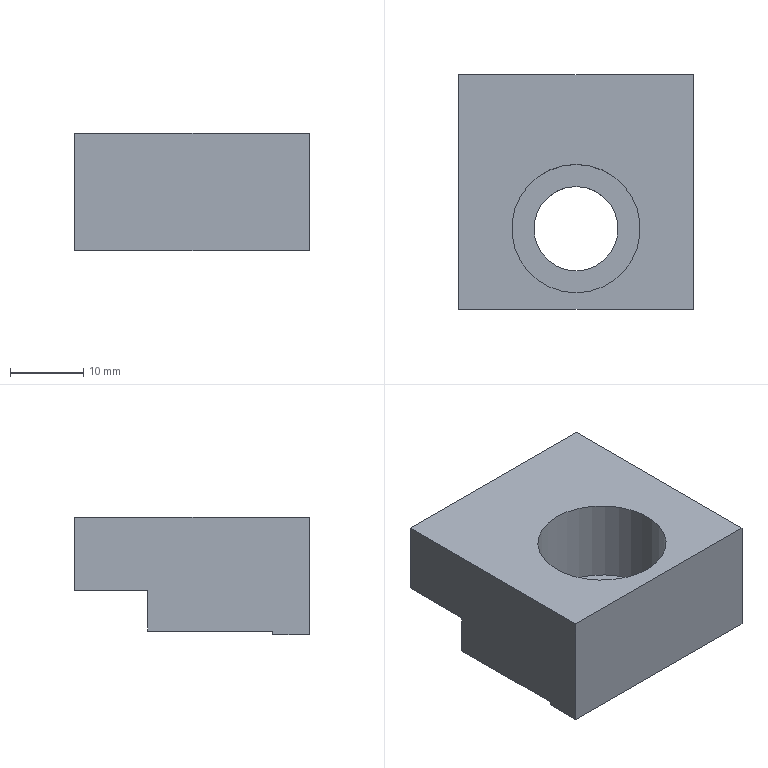Part | NX | features MAIN_BODY 2 | 1 solid | 13 faces | box 32 x 32 x 16 mm | volume 11010 mm3 | plane 11 | cylinder 2 | commonest cylinder face diameters 11.5 x1 17.5 x1
STEP:
#1=CARTESIAN_POINT('',(-279.,-369.5,260.));
#2=VERTEX_POINT('',#1);
#3=CARTESIAN_POINT('',(-279.,-369.5,276.));
#4=VERTEX_POINT('',#3);
#5=CARTESIAN_POINT('',(-279.,-369.5,260.));
#6=DIRECTION('',(0.,0.,-1.));
#7=VECTOR('',#6,1000.);
#8=LINE('',#5,#7);
#9=EDGE_CURVE('',#2,#4,#8,.F.);
#10=ORIENTED_EDGE('',*,*,#9,.F.);
#11=CARTESIAN_POINT('',(-279.,-364.5,260.));
#12=VERTEX_POINT('',#11);
#13=CARTESIAN_POINT('',(-279.,-357.5,260.));
#14=DIRECTION('',(0.,1.,0.));
#15=VECTOR('',#14,1000.);
#16=LINE('',#13,#15);
#17=EDGE_CURVE('',#2,#12,#16,.T.);
#18=ORIENTED_EDGE('',*,*,#17,.T.);
#19=CARTESIAN_POINT('',(-279.,-364.5,260.5));
#20=VERTEX_POINT('',#19);
#21=CARTESIAN_POINT('',(-279.,-364.5,260.));
#22=DIRECTION('',(0.,0.,-1.));
#23=VECTOR('',#22,1000.);
#24=LINE('',#21,#23);
#25=EDGE_CURVE('',#12,#20,#24,.F.);
#26=ORIENTED_EDGE('',*,*,#25,.T.);
#27=CARTESIAN_POINT('',(-279.,-347.5,260.5));
#28=VERTEX_POINT('',#27);
#29=CARTESIAN_POINT('',(-279.,-347.5,260.5));
#30=DIRECTION('',(0.,1.,0.));
#31=VECTOR('',#30,1000.);
#32=LINE('',#29,#31);
#33=EDGE_CURVE('',#28,#20,#32,.F.);
#34=ORIENTED_EDGE('',*,*,#33,.F.);
#35=CARTESIAN_POINT('',(-279.,-347.5,266.));
#36=VERTEX_POINT('',#35);
#37=CARTESIAN_POINT('',(-279.,-347.5,260.));
#38=DIRECTION('',(0.,0.,-1.));
#39=VECTOR('',#38,1000.);
#40=LINE('',#37,#39);
#41=EDGE_CURVE('',#28,#36,#40,.F.);
#42=ORIENTED_EDGE('',*,*,#41,.T.);
#43=CARTESIAN_POINT('',(-279.,-337.5,266.));
#44=VERTEX_POINT('',#43);
#45=CARTESIAN_POINT('',(-279.,-357.5,266.));
#46=DIRECTION('',(0.,-1.,0.));
#47=VECTOR('',#46,1000.);
#48=LINE('',#45,#47);
#49=EDGE_CURVE('',#44,#36,#48,.T.);
#50=ORIENTED_EDGE('',*,*,#49,.F.);
#51=CARTESIAN_POINT('',(-279.,-337.5,276.));
#52=VERTEX_POINT('',#51);
#53=CARTESIAN_POINT('',(-279.,-337.5,260.));
#54=DIRECTION('',(0.,0.,-1.));
#55=VECTOR('',#54,1000.);
#56=LINE('',#53,#55);
#57=EDGE_CURVE('',#44,#52,#56,.F.);
#58=ORIENTED_EDGE('',*,*,#57,.T.);
#59=CARTESIAN_POINT('',(-279.,-357.5,276.));
#60=DIRECTION('',(0.,-1.,0.));
#61=VECTOR('',#60,1000.);
#62=LINE('',#59,#61);
#63=EDGE_CURVE('',#4,#52,#62,.F.);
#64=ORIENTED_EDGE('',*,*,#63,.F.);
#65=EDGE_LOOP('',(#10,#18,#26,#34,#42,#50,#58,#64));
#66=FACE_BOUND('',#65,.T.);
#67=CARTESIAN_POINT('',(-279.,-357.5,260.));
#68=DIRECTION('',(1.,0.,0.));
#69=DIRECTION('',(0.,0.,1.));
#70=AXIS2_PLACEMENT_3D('',#67,#68,#69);
#71=PLANE('',#70);
#72=ADVANCED_FACE('',(#66),#71,.T.);
#73=CARTESIAN_POINT('',(-311.,-369.5,276.));
#74=VERTEX_POINT('',#73);
#75=CARTESIAN_POINT('',(-311.,-337.5,276.));
#76=VERTEX_POINT('',#75);
#77=CARTESIAN_POINT('',(-311.,-357.5,276.));
#78=DIRECTION('',(0.,1.,0.));
#79=VECTOR('',#78,1000.);
#80=LINE('',#77,#79);
#81=EDGE_CURVE('',#74,#76,#80,.T.);
#82=ORIENTED_EDGE('',*,*,#81,.T.);
#83=CARTESIAN_POINT('',(-311.,-337.5,266.));
#84=VERTEX_POINT('',#83);
#85=CARTESIAN_POINT('',(-311.,-337.5,260.));
#86=DIRECTION('',(0.,0.,1.));
#87=VECTOR('',#86,1000.);
#88=LINE('',#85,#87);
#89=EDGE_CURVE('',#84,#76,#88,.T.);
#90=ORIENTED_EDGE('',*,*,#89,.F.);
#91=CARTESIAN_POINT('',(-311.,-347.5,266.));
#92=VERTEX_POINT('',#91);
#93=CARTESIAN_POINT('',(-311.,-337.5,266.));
#94=DIRECTION('',(0.,1.,0.));
#95=VECTOR('',#94,1000.);
#96=LINE('',#93,#95);
#97=EDGE_CURVE('',#84,#92,#96,.F.);
#98=ORIENTED_EDGE('',*,*,#97,.T.);
#99=CARTESIAN_POINT('',(-311.,-347.5,260.5));
#100=VERTEX_POINT('',#99);
#101=CARTESIAN_POINT('',(-311.,-347.5,260.));
#102=DIRECTION('',(0.,0.,1.));
#103=VECTOR('',#102,1000.);
#104=LINE('',#101,#103);
#105=EDGE_CURVE('',#100,#92,#104,.T.);
#106=ORIENTED_EDGE('',*,*,#105,.F.);
#107=CARTESIAN_POINT('',(-311.,-364.5,260.5));
#108=VERTEX_POINT('',#107);
#109=CARTESIAN_POINT('',(-311.,-357.5,260.5));
#110=DIRECTION('',(0.,-1.,0.));
#111=VECTOR('',#110,1000.);
#112=LINE('',#109,#111);
#113=EDGE_CURVE('',#100,#108,#112,.T.);
#114=ORIENTED_EDGE('',*,*,#113,.T.);
#115=CARTESIAN_POINT('',(-311.,-364.5,260.));
#116=VERTEX_POINT('',#115);
#117=CARTESIAN_POINT('',(-311.,-364.5,260.));
#118=DIRECTION('',(0.,0.,1.));
#119=VECTOR('',#118,1000.);
#120=LINE('',#117,#119);
#121=EDGE_CURVE('',#116,#108,#120,.T.);
#122=ORIENTED_EDGE('',*,*,#121,.F.);
#123=CARTESIAN_POINT('',(-311.,-369.5,260.));
#124=VERTEX_POINT('',#123);
#125=CARTESIAN_POINT('',(-311.,-357.5,260.));
#126=DIRECTION('',(0.,-1.,0.));
#127=VECTOR('',#126,1000.);
#128=LINE('',#125,#127);
#129=EDGE_CURVE('',#124,#116,#128,.F.);
#130=ORIENTED_EDGE('',*,*,#129,.F.);
#131=CARTESIAN_POINT('',(-311.,-369.5,260.));
#132=DIRECTION('',(0.,0.,1.));
#133=VECTOR('',#132,1000.);
#134=LINE('',#131,#133);
#135=EDGE_CURVE('',#124,#74,#134,.T.);
#136=ORIENTED_EDGE('',*,*,#135,.T.);
#137=EDGE_LOOP('',(#82,#90,#98,#106,#114,#122,#130,#136));
#138=FACE_BOUND('',#137,.T.);
#139=CARTESIAN_POINT('',(-311.,-357.5,260.));
#140=DIRECTION('',(1.,0.,0.));
#141=DIRECTION('',(0.,0.,1.));
#142=AXIS2_PLACEMENT_3D('',#139,#140,#141);
#143=PLANE('',#142);
#144=ADVANCED_FACE('',(#138),#143,.F.);
#145=ORIENTED_EDGE('',*,*,#41,.F.);
#146=CARTESIAN_POINT('',(-305.,-347.5,260.5));
#147=DIRECTION('',(1.,0.,0.));
#148=VECTOR('',#147,1000.);
#149=LINE('',#146,#148);
#150=EDGE_CURVE('',#100,#28,#149,.T.);
#151=ORIENTED_EDGE('',*,*,#150,.F.);
#152=ORIENTED_EDGE('',*,*,#105,.T.);
#153=CARTESIAN_POINT('',(-305.,-347.5,266.));
#154=DIRECTION('',(-1.,0.,0.));
#155=VECTOR('',#154,1000.);
#156=LINE('',#153,#155);
#157=EDGE_CURVE('',#92,#36,#156,.F.);
#158=ORIENTED_EDGE('',*,*,#157,.T.);
#159=EDGE_LOOP('',(#145,#151,#152,#158));
#160=FACE_BOUND('',#159,.T.);
#161=CARTESIAN_POINT('',(-305.,-347.5,260.));
#162=DIRECTION('',(0.,-1.,0.));
#163=DIRECTION('',(0.,0.,-1.));
#164=AXIS2_PLACEMENT_3D('',#161,#162,#163);
#165=PLANE('',#164);
#166=ADVANCED_FACE('',(#160),#165,.F.);
#167=ORIENTED_EDGE('',*,*,#129,.T.);
#168=CARTESIAN_POINT('',(-305.,-364.5,260.));
#169=DIRECTION('',(-1.,0.,0.));
#170=VECTOR('',#169,1000.);
#171=LINE('',#168,#170);
#172=EDGE_CURVE('',#116,#12,#171,.F.);
#173=ORIENTED_EDGE('',*,*,#172,.T.);
#174=ORIENTED_EDGE('',*,*,#17,.F.);
#175=CARTESIAN_POINT('',(-305.,-369.5,260.));
#176=DIRECTION('',(-1.,0.,0.));
#177=VECTOR('',#176,1000.);
#178=LINE('',#175,#177);
#179=EDGE_CURVE('',#124,#2,#178,.F.);
#180=ORIENTED_EDGE('',*,*,#179,.F.);
#181=EDGE_LOOP('',(#167,#173,#174,#180));
#182=FACE_BOUND('',#181,.T.);
#183=CARTESIAN_POINT('',(-305.,-357.5,260.));
#184=DIRECTION('',(0.,0.,-1.));
#185=DIRECTION('',(1.,0.,0.));
#186=AXIS2_PLACEMENT_3D('',#183,#184,#185);
#187=PLANE('',#186);
#188=ADVANCED_FACE('',(#182),#187,.T.);
#189=CARTESIAN_POINT('',(-295.,-367.25,276.));
#190=VERTEX_POINT('',#189);
#191=CARTESIAN_POINT('',(-295.,-358.5,276.));
#192=DIRECTION('',(0.,0.,1.));
#193=DIRECTION('',(0.,-1.,0.));
#194=AXIS2_PLACEMENT_3D('',#191,#192,#193);
#195=CIRCLE('',#194,8.75);
#196=EDGE_CURVE('',#190,#190,#195,.T.);
#197=ORIENTED_EDGE('',*,*,#196,.F.);
#198=EDGE_LOOP('',(#197));
#199=FACE_BOUND('',#198,.T.);
#200=CARTESIAN_POINT('',(-305.,-337.5,276.));
#201=DIRECTION('',(1.,0.,0.));
#202=VECTOR('',#201,1000.);
#203=LINE('',#200,#202);
#204=EDGE_CURVE('',#76,#52,#203,.T.);
#205=ORIENTED_EDGE('',*,*,#204,.F.);
#206=ORIENTED_EDGE('',*,*,#81,.F.);
#207=CARTESIAN_POINT('',(-305.,-369.5,276.));
#208=DIRECTION('',(1.,0.,0.));
#209=VECTOR('',#208,1000.);
#210=LINE('',#207,#209);
#211=EDGE_CURVE('',#74,#4,#210,.T.);
#212=ORIENTED_EDGE('',*,*,#211,.T.);
#213=ORIENTED_EDGE('',*,*,#63,.T.);
#214=EDGE_LOOP('',(#205,#206,#212,#213));
#215=FACE_BOUND('',#214,.T.);
#216=CARTESIAN_POINT('',(-305.,-357.5,276.));
#217=DIRECTION('',(0.,0.,-1.));
#218=DIRECTION('',(1.,0.,0.));
#219=AXIS2_PLACEMENT_3D('',#216,#217,#218);
#220=PLANE('',#219);
#221=ADVANCED_FACE('',(#199,#215),#220,.F.);
#222=CARTESIAN_POINT('',(-305.,-337.5,266.));
#223=DIRECTION('',(-1.,0.,0.));
#224=VECTOR('',#223,1000.);
#225=LINE('',#222,#224);
#226=EDGE_CURVE('',#84,#44,#225,.F.);
#227=ORIENTED_EDGE('',*,*,#226,.F.);
#228=ORIENTED_EDGE('',*,*,#89,.T.);
#229=ORIENTED_EDGE('',*,*,#204,.T.);
#230=ORIENTED_EDGE('',*,*,#57,.F.);
#231=EDGE_LOOP('',(#227,#228,#229,#230));
#232=FACE_BOUND('',#231,.T.);
#233=CARTESIAN_POINT('',(-305.,-337.5,260.));
#234=DIRECTION('',(0.,-1.,0.));
#235=DIRECTION('',(0.,0.,-1.));
#236=AXIS2_PLACEMENT_3D('',#233,#234,#235);
#237=PLANE('',#236);
#238=ADVANCED_FACE('',(#232),#237,.F.);
#239=ORIENTED_EDGE('',*,*,#211,.F.);
#240=ORIENTED_EDGE('',*,*,#135,.F.);
#241=ORIENTED_EDGE('',*,*,#179,.T.);
#242=ORIENTED_EDGE('',*,*,#9,.T.);
#243=EDGE_LOOP('',(#239,#240,#241,#242));
#244=FACE_BOUND('',#243,.T.);
#245=CARTESIAN_POINT('',(-305.,-369.5,260.));
#246=DIRECTION('',(0.,-1.,0.));
#247=DIRECTION('',(0.,0.,-1.));
#248=AXIS2_PLACEMENT_3D('',#245,#246,#247);
#249=PLANE('',#248);
#250=ADVANCED_FACE('',(#244),#249,.T.);
#251=ORIENTED_EDGE('',*,*,#157,.F.);
#252=ORIENTED_EDGE('',*,*,#97,.F.);
#253=ORIENTED_EDGE('',*,*,#226,.T.);
#254=ORIENTED_EDGE('',*,*,#49,.T.);
#255=EDGE_LOOP('',(#251,#252,#253,#254));
#256=FACE_BOUND('',#255,.T.);
#257=CARTESIAN_POINT('',(-305.,-337.5,266.));
#258=DIRECTION('',(0.,0.,-1.));
#259=DIRECTION('',(1.,0.,0.));
#260=AXIS2_PLACEMENT_3D('',#257,#258,#259);
#261=PLANE('',#260);
#262=ADVANCED_FACE('',(#256),#261,.T.);
#263=CARTESIAN_POINT('',(-295.,-364.25,260.5));
#264=VERTEX_POINT('',#263);
#265=CARTESIAN_POINT('',(-295.,-358.5,260.5));
#266=DIRECTION('',(0.,0.,1.));
#267=DIRECTION('',(0.,-1.,0.));
#268=AXIS2_PLACEMENT_3D('',#265,#266,#267);
#269=CIRCLE('',#268,5.75);
#270=EDGE_CURVE('',#264,#264,#269,.T.);
#271=ORIENTED_EDGE('',*,*,#270,.T.);
#272=EDGE_LOOP('',(#271));
#273=FACE_BOUND('',#272,.T.);
#274=ORIENTED_EDGE('',*,*,#33,.T.);
#275=CARTESIAN_POINT('',(-305.,-364.5,260.5));
#276=DIRECTION('',(1.,0.,0.));
#277=VECTOR('',#276,1000.);
#278=LINE('',#275,#277);
#279=EDGE_CURVE('',#108,#20,#278,.T.);
#280=ORIENTED_EDGE('',*,*,#279,.F.);
#281=ORIENTED_EDGE('',*,*,#113,.F.);
#282=ORIENTED_EDGE('',*,*,#150,.T.);
#283=EDGE_LOOP('',(#274,#280,#281,#282));
#284=FACE_BOUND('',#283,.T.);
#285=CARTESIAN_POINT('',(-305.,-347.5,260.5));
#286=DIRECTION('',(0.,0.,-1.));
#287=DIRECTION('',(1.,0.,0.));
#288=AXIS2_PLACEMENT_3D('',#285,#286,#287);
#289=PLANE('',#288);
#290=ADVANCED_FACE('',(#273,#284),#289,.T.);
#291=ORIENTED_EDGE('',*,*,#172,.F.);
#292=ORIENTED_EDGE('',*,*,#121,.T.);
#293=ORIENTED_EDGE('',*,*,#279,.T.);
#294=ORIENTED_EDGE('',*,*,#25,.F.);
#295=EDGE_LOOP('',(#291,#292,#293,#294));
#296=FACE_BOUND('',#295,.T.);
#297=CARTESIAN_POINT('',(-305.,-364.5,260.));
#298=DIRECTION('',(0.,-1.,0.));
#299=DIRECTION('',(0.,0.,-1.));
#300=AXIS2_PLACEMENT_3D('',#297,#298,#299);
#301=PLANE('',#300);
#302=ADVANCED_FACE('',(#296),#301,.F.);
#303=ORIENTED_EDGE('',*,*,#270,.F.);
#304=EDGE_LOOP('',(#303));
#305=FACE_BOUND('',#304,.T.);
#306=CARTESIAN_POINT('',(-295.,-364.25,264.5));
#307=VERTEX_POINT('',#306);
#308=CARTESIAN_POINT('',(-295.,-358.5,264.5));
#309=DIRECTION('',(0.,0.,1.));
#310=DIRECTION('',(0.,-1.,0.));
#311=AXIS2_PLACEMENT_3D('',#308,#309,#310);
#312=CIRCLE('',#311,5.75);
#313=EDGE_CURVE('',#307,#307,#312,.T.);
#314=ORIENTED_EDGE('',*,*,#313,.T.);
#315=EDGE_LOOP('',(#314));
#316=FACE_BOUND('',#315,.T.);
#317=CARTESIAN_POINT('',(-295.,-358.5,226.));
#318=DIRECTION('',(0.,0.,-1.));
#319=DIRECTION('',(0.,-1.,0.));
#320=AXIS2_PLACEMENT_3D('',#317,#318,#319);
#321=CYLINDRICAL_SURFACE('',#320,5.75);
#322=ADVANCED_FACE('',(#305,#316),#321,.F.);
#323=ORIENTED_EDGE('',*,*,#313,.F.);
#324=EDGE_LOOP('',(#323));
#325=FACE_BOUND('',#324,.T.);
#326=CARTESIAN_POINT('',(-295.,-367.25,264.5));
#327=VERTEX_POINT('',#326);
#328=CARTESIAN_POINT('',(-295.,-358.5,264.5));
#329=DIRECTION('',(0.,0.,1.));
#330=DIRECTION('',(0.,-1.,0.));
#331=AXIS2_PLACEMENT_3D('',#328,#329,#330);
#332=CIRCLE('',#331,8.75);
#333=EDGE_CURVE('',#327,#327,#332,.T.);
#334=ORIENTED_EDGE('',*,*,#333,.T.);
#335=EDGE_LOOP('',(#334));
#336=FACE_BOUND('',#335,.T.);
#337=CARTESIAN_POINT('',(-295.,-358.5,264.5));
#338=DIRECTION('',(0.,0.,-1.));
#339=DIRECTION('',(0.,-1.,0.));
#340=AXIS2_PLACEMENT_3D('',#337,#338,#339);
#341=PLANE('',#340);
#342=ADVANCED_FACE('',(#325,#336),#341,.F.);
#343=ORIENTED_EDGE('',*,*,#333,.F.);
#344=EDGE_LOOP('',(#343));
#345=FACE_BOUND('',#344,.T.);
#346=ORIENTED_EDGE('',*,*,#196,.T.);
#347=EDGE_LOOP('',(#346));
#348=FACE_BOUND('',#347,.T.);
#349=CARTESIAN_POINT('',(-295.,-358.5,276.));
#350=DIRECTION('',(0.,0.,-1.));
#351=DIRECTION('',(0.,-1.,0.));
#352=AXIS2_PLACEMENT_3D('',#349,#350,#351);
#353=CYLINDRICAL_SURFACE('',#352,8.75);
#354=ADVANCED_FACE('',(#345,#348),#353,.F.);
#355=CLOSED_SHELL('',(#72,#144,#166,#188,#221,#238,#250,#262,#290,#302,#322,#342,#354));
#356=MANIFOLD_SOLID_BREP('',#355);
#357=(LENGTH_UNIT()NAMED_UNIT(*)SI_UNIT(.MILLI.,.METRE.));
#358=UNCERTAINTY_MEASURE_WITH_UNIT(LENGTH_MEASURE(0.00001),#357,'','');
#359=(NAMED_UNIT(*)PLANE_ANGLE_UNIT()SI_UNIT($,.RADIAN.));
#360=(NAMED_UNIT(*)SI_UNIT($,.STERADIAN.)SOLID_ANGLE_UNIT());
#361=(GEOMETRIC_REPRESENTATION_CONTEXT(3)GLOBAL_UNCERTAINTY_ASSIGNED_CONTEXT((#358))GLOBAL_UNIT_ASSIGNED_CONTEXT((#357,#359,#360))REPRESENTATION_CONTEXT('',''));
#362=ADVANCED_BREP_SHAPE_REPRESENTATION('',(#356),#361);